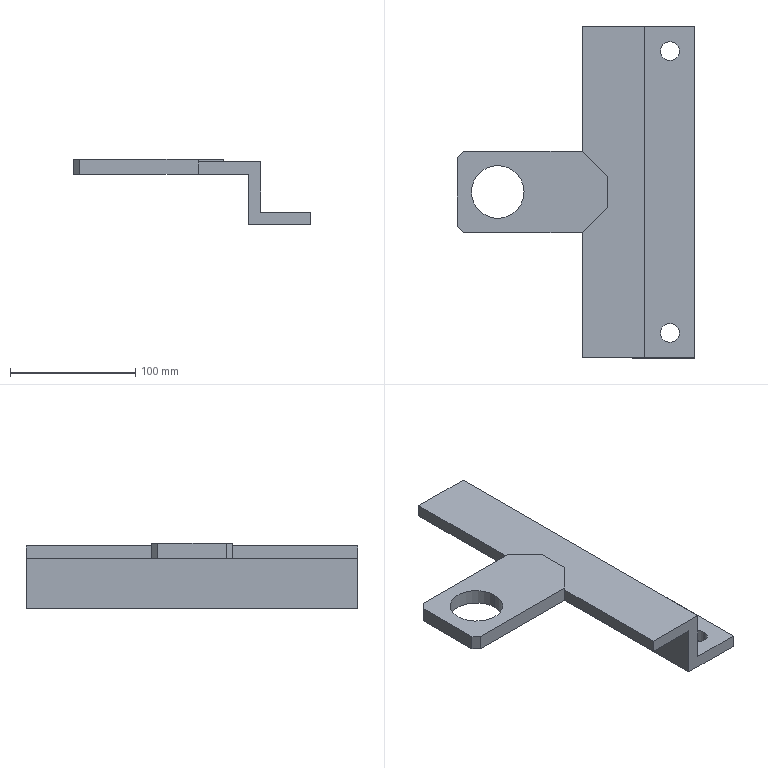Part | SolidWorks | features ICE 4, Chamfer 2, Extrusion 1 | 1 solid | 26 faces | box 190 x 265 x 52 mm | volume 403840 mm3 | plane 20 | cylinder 6 | commonest cylinder face diameters 15 x4 42 x2
STEP:
#1=CARTESIAN_POINT('',(130.,112.5,-40.));
#2=VERTEX_POINT('',#1);
#3=CARTESIAN_POINT('',(145.,112.5,-40.));
#4=VERTEX_POINT('',#3);
#5=CARTESIAN_POINT('',(137.5,112.5,-40.));
#6=DIRECTION('',(0.,0.,1.));
#7=DIRECTION('',(1.,0.,0.));
#8=AXIS2_PLACEMENT_3D('',#5,#6,#7);
#9=CIRCLE('',#8,7.5);
#10=EDGE_CURVE('',#2,#4,#9,.T.);
#11=ORIENTED_EDGE('',*,*,#10,.F.);
#12=CARTESIAN_POINT('',(130.,112.5,-30.));
#13=VERTEX_POINT('',#12);
#14=CARTESIAN_POINT('',(130.,112.5,-40.));
#15=DIRECTION('',(0.,0.,1.));
#16=VECTOR('',#15,1000.);
#17=LINE('',#14,#16);
#18=EDGE_CURVE('',#2,#13,#17,.T.);
#19=ORIENTED_EDGE('',*,*,#18,.T.);
#20=CARTESIAN_POINT('',(145.,112.5,-30.));
#21=VERTEX_POINT('',#20);
#22=CARTESIAN_POINT('',(137.5,112.5,-30.));
#23=DIRECTION('',(0.,0.,1.));
#24=DIRECTION('',(1.,0.,0.));
#25=AXIS2_PLACEMENT_3D('',#22,#23,#24);
#26=CIRCLE('',#25,7.5);
#27=EDGE_CURVE('',#13,#21,#26,.T.);
#28=ORIENTED_EDGE('',*,*,#27,.T.);
#29=CARTESIAN_POINT('',(145.,112.5,-40.));
#30=DIRECTION('',(0.,0.,1.));
#31=VECTOR('',#30,1000.);
#32=LINE('',#29,#31);
#33=EDGE_CURVE('',#4,#21,#32,.T.);
#34=ORIENTED_EDGE('',*,*,#33,.F.);
#35=EDGE_LOOP('',(#11,#19,#28,#34));
#36=FACE_OUTER_BOUND('',#35,.T.);
#37=CARTESIAN_POINT('',(137.5,112.5,-40.));
#38=DIRECTION('',(0.,0.,1.));
#39=DIRECTION('',(1.,0.,0.));
#40=AXIS2_PLACEMENT_3D('',#37,#38,#39);
#41=CYLINDRICAL_SURFACE('',#40,7.5);
#42=ADVANCED_FACE('',(#36),#41,.F.);
#43=CARTESIAN_POINT('',(130.,-112.5,-40.));
#44=VERTEX_POINT('',#43);
#45=CARTESIAN_POINT('',(145.,-112.5,-40.));
#46=VERTEX_POINT('',#45);
#47=CARTESIAN_POINT('',(137.5,-112.5,-40.));
#48=DIRECTION('',(0.,0.,1.));
#49=DIRECTION('',(1.,0.,0.));
#50=AXIS2_PLACEMENT_3D('',#47,#48,#49);
#51=CIRCLE('',#50,7.5);
#52=EDGE_CURVE('',#44,#46,#51,.T.);
#53=ORIENTED_EDGE('',*,*,#52,.F.);
#54=CARTESIAN_POINT('',(130.,-112.5,-30.));
#55=VERTEX_POINT('',#54);
#56=CARTESIAN_POINT('',(130.,-112.5,-40.));
#57=DIRECTION('',(0.,0.,1.));
#58=VECTOR('',#57,1000.);
#59=LINE('',#56,#58);
#60=EDGE_CURVE('',#44,#55,#59,.T.);
#61=ORIENTED_EDGE('',*,*,#60,.T.);
#62=CARTESIAN_POINT('',(145.,-112.5,-30.));
#63=VERTEX_POINT('',#62);
#64=CARTESIAN_POINT('',(137.5,-112.5,-30.));
#65=DIRECTION('',(0.,0.,1.));
#66=DIRECTION('',(1.,0.,0.));
#67=AXIS2_PLACEMENT_3D('',#64,#65,#66);
#68=CIRCLE('',#67,7.5);
#69=EDGE_CURVE('',#55,#63,#68,.T.);
#70=ORIENTED_EDGE('',*,*,#69,.T.);
#71=CARTESIAN_POINT('',(145.,-112.5,-40.));
#72=DIRECTION('',(0.,0.,1.));
#73=VECTOR('',#72,1000.);
#74=LINE('',#71,#73);
#75=EDGE_CURVE('',#46,#63,#74,.T.);
#76=ORIENTED_EDGE('',*,*,#75,.F.);
#77=EDGE_LOOP('',(#53,#61,#70,#76));
#78=FACE_OUTER_BOUND('',#77,.T.);
#79=CARTESIAN_POINT('',(137.5,-112.5,-40.));
#80=DIRECTION('',(0.,0.,1.));
#81=DIRECTION('',(1.,0.,0.));
#82=AXIS2_PLACEMENT_3D('',#79,#80,#81);
#83=CYLINDRICAL_SURFACE('',#82,7.5);
#84=ADVANCED_FACE('',(#78),#83,.F.);
#85=CARTESIAN_POINT('',(-21.,0.,12.));
#86=VERTEX_POINT('',#85);
#87=CARTESIAN_POINT('',(21.,0.,12.));
#88=VERTEX_POINT('',#87);
#89=CARTESIAN_POINT('',(0.,0.,12.));
#90=DIRECTION('',(0.,0.,1.));
#91=DIRECTION('',(1.,0.,0.));
#92=AXIS2_PLACEMENT_3D('',#89,#90,#91);
#93=CIRCLE('',#92,21.);
#94=EDGE_CURVE('',#86,#88,#93,.T.);
#95=ORIENTED_EDGE('',*,*,#94,.T.);
#96=CARTESIAN_POINT('',(21.,0.,0.));
#97=VERTEX_POINT('',#96);
#98=CARTESIAN_POINT('',(21.,0.,12.));
#99=DIRECTION('',(0.,0.,-1.));
#100=VECTOR('',#99,1000.);
#101=LINE('',#98,#100);
#102=EDGE_CURVE('',#88,#97,#101,.T.);
#103=ORIENTED_EDGE('',*,*,#102,.T.);
#104=CARTESIAN_POINT('',(-21.,0.,0.));
#105=VERTEX_POINT('',#104);
#106=CARTESIAN_POINT('',(0.,0.,0.));
#107=DIRECTION('',(0.,0.,1.));
#108=DIRECTION('',(1.,0.,0.));
#109=AXIS2_PLACEMENT_3D('',#106,#107,#108);
#110=CIRCLE('',#109,21.);
#111=EDGE_CURVE('',#105,#97,#110,.T.);
#112=ORIENTED_EDGE('',*,*,#111,.F.);
#113=CARTESIAN_POINT('',(-21.,0.,12.));
#114=DIRECTION('',(0.,0.,-1.));
#115=VECTOR('',#114,1000.);
#116=LINE('',#113,#115);
#117=EDGE_CURVE('',#86,#105,#116,.T.);
#118=ORIENTED_EDGE('',*,*,#117,.F.);
#119=EDGE_LOOP('',(#95,#103,#112,#118));
#120=FACE_OUTER_BOUND('',#119,.T.);
#121=CARTESIAN_POINT('',(0.,0.,12.));
#122=DIRECTION('',(0.,0.,-1.));
#123=DIRECTION('',(-1.,0.,0.));
#124=AXIS2_PLACEMENT_3D('',#121,#122,#123);
#125=CYLINDRICAL_SURFACE('',#124,21.);
#126=ADVANCED_FACE('',(#120),#125,.F.);
#127=CARTESIAN_POINT('',(117.5,-132.5,10.));
#128=VERTEX_POINT('',#127);
#129=CARTESIAN_POINT('',(117.5,-132.5,-30.));
#130=VERTEX_POINT('',#129);
#131=CARTESIAN_POINT('',(117.5,-132.5,10.));
#132=DIRECTION('',(0.,0.,-1.));
#133=VECTOR('',#132,1000.);
#134=LINE('',#131,#133);
#135=EDGE_CURVE('',#128,#130,#134,.T.);
#136=ORIENTED_EDGE('',*,*,#135,.T.);
#137=CARTESIAN_POINT('',(117.5,132.5,-30.));
#138=VERTEX_POINT('',#137);
#139=CARTESIAN_POINT('',(117.5,-132.5,-30.));
#140=DIRECTION('',(0.,1.,0.));
#141=VECTOR('',#140,1000.);
#142=LINE('',#139,#141);
#143=EDGE_CURVE('',#130,#138,#142,.T.);
#144=ORIENTED_EDGE('',*,*,#143,.T.);
#145=CARTESIAN_POINT('',(117.5,132.5,10.));
#146=VERTEX_POINT('',#145);
#147=CARTESIAN_POINT('',(117.5,132.5,10.));
#148=DIRECTION('',(0.,0.,-1.));
#149=VECTOR('',#148,1000.);
#150=LINE('',#147,#149);
#151=EDGE_CURVE('',#146,#138,#150,.T.);
#152=ORIENTED_EDGE('',*,*,#151,.F.);
#153=CARTESIAN_POINT('',(117.5,-132.5,10.));
#154=DIRECTION('',(0.,-1.,0.));
#155=VECTOR('',#154,1000.);
#156=LINE('',#153,#155);
#157=EDGE_CURVE('',#146,#128,#156,.T.);
#158=ORIENTED_EDGE('',*,*,#157,.T.);
#159=EDGE_LOOP('',(#136,#144,#152,#158));
#160=FACE_OUTER_BOUND('',#159,.T.);
#161=CARTESIAN_POINT('',(117.5,-132.5,10.));
#162=DIRECTION('',(1.,0.,0.));
#163=DIRECTION('',(0.,0.,-1.));
#164=AXIS2_PLACEMENT_3D('',#161,#162,#163);
#165=PLANE('',#164);
#166=ADVANCED_FACE('',(#160),#165,.T.);
#167=CARTESIAN_POINT('',(87.5,-12.5,12.));
#168=VERTEX_POINT('',#167);
#169=CARTESIAN_POINT('',(87.5,12.5,12.));
#170=VERTEX_POINT('',#169);
#171=CARTESIAN_POINT('',(87.5,32.5,12.));
#172=DIRECTION('',(0.,1.,0.));
#173=VECTOR('',#172,1000.);
#174=LINE('',#171,#173);
#175=EDGE_CURVE('',#168,#170,#174,.T.);
#176=ORIENTED_EDGE('',*,*,#175,.T.);
#177=CARTESIAN_POINT('',(67.5,32.5,12.));
#178=VERTEX_POINT('',#177);
#179=CARTESIAN_POINT('',(50.,50.,12.));
#180=DIRECTION('',(-0.7071,0.7071,0.));
#181=VECTOR('',#180,1000.);
#182=LINE('',#179,#181);
#183=EDGE_CURVE('',#170,#178,#182,.T.);
#184=ORIENTED_EDGE('',*,*,#183,.T.);
#185=CARTESIAN_POINT('',(-27.5,32.5,12.));
#186=VERTEX_POINT('',#185);
#187=CARTESIAN_POINT('',(32.5,32.5,12.));
#188=DIRECTION('',(-1.,0.,0.));
#189=VECTOR('',#188,1000.);
#190=LINE('',#187,#189);
#191=EDGE_CURVE('',#178,#186,#190,.T.);
#192=ORIENTED_EDGE('',*,*,#191,.T.);
#193=CARTESIAN_POINT('',(-32.5,27.5,12.));
#194=VERTEX_POINT('',#193);
#195=CARTESIAN_POINT('',(-30.,30.,12.));
#196=DIRECTION('',(-0.7071,-0.7071,0.));
#197=VECTOR('',#196,1000.);
#198=LINE('',#195,#197);
#199=EDGE_CURVE('',#186,#194,#198,.T.);
#200=ORIENTED_EDGE('',*,*,#199,.T.);
#201=CARTESIAN_POINT('',(-32.5,-27.5,12.));
#202=VERTEX_POINT('',#201);
#203=CARTESIAN_POINT('',(-32.5,32.5,12.));
#204=DIRECTION('',(0.,-1.,0.));
#205=VECTOR('',#204,1000.);
#206=LINE('',#203,#205);
#207=EDGE_CURVE('',#194,#202,#206,.T.);
#208=ORIENTED_EDGE('',*,*,#207,.T.);
#209=CARTESIAN_POINT('',(-27.5,-32.5,12.));
#210=VERTEX_POINT('',#209);
#211=CARTESIAN_POINT('',(-30.,-30.,12.));
#212=DIRECTION('',(0.7071,-0.7071,0.));
#213=VECTOR('',#212,1000.);
#214=LINE('',#211,#213);
#215=EDGE_CURVE('',#202,#210,#214,.T.);
#216=ORIENTED_EDGE('',*,*,#215,.T.);
#217=CARTESIAN_POINT('',(67.5,-32.5,12.));
#218=VERTEX_POINT('',#217);
#219=CARTESIAN_POINT('',(87.5,-32.5,12.));
#220=DIRECTION('',(1.,0.,0.));
#221=VECTOR('',#220,1000.);
#222=LINE('',#219,#221);
#223=EDGE_CURVE('',#210,#218,#222,.T.);
#224=ORIENTED_EDGE('',*,*,#223,.T.);
#225=CARTESIAN_POINT('',(50.,-50.,12.));
#226=DIRECTION('',(0.7071,0.7071,0.));
#227=VECTOR('',#226,1000.);
#228=LINE('',#225,#227);
#229=EDGE_CURVE('',#218,#168,#228,.T.);
#230=ORIENTED_EDGE('',*,*,#229,.T.);
#231=EDGE_LOOP('',(#176,#184,#192,#200,#208,#216,#224,#230));
#232=FACE_OUTER_BOUND('',#231,.T.);
#233=ORIENTED_EDGE('',*,*,#94,.F.);
#234=CARTESIAN_POINT('',(0.,0.,12.));
#235=DIRECTION('',(0.,0.,1.));
#236=DIRECTION('',(1.,0.,0.));
#237=AXIS2_PLACEMENT_3D('',#234,#235,#236);
#238=CIRCLE('',#237,21.);
#239=EDGE_CURVE('',#88,#86,#238,.T.);
#240=ORIENTED_EDGE('',*,*,#239,.F.);
#241=EDGE_LOOP('',(#233,#240));
#242=FACE_BOUND('',#241,.T.);
#243=CARTESIAN_POINT('',(0.,0.,12.));
#244=DIRECTION('',(0.,0.,1.));
#245=DIRECTION('',(1.,0.,0.));
#246=AXIS2_PLACEMENT_3D('',#243,#244,#245);
#247=PLANE('',#246);
#248=ADVANCED_FACE('',(#232,#242),#247,.T.);
#249=CARTESIAN_POINT('',(67.5,132.5,0.));
#250=VERTEX_POINT('',#249);
#251=CARTESIAN_POINT('',(107.5,132.5,0.));
#252=VERTEX_POINT('',#251);
#253=CARTESIAN_POINT('',(117.5,132.5,0.));
#254=DIRECTION('',(1.,0.,0.));
#255=VECTOR('',#254,1000.);
#256=LINE('',#253,#255);
#257=EDGE_CURVE('',#250,#252,#256,.T.);
#258=ORIENTED_EDGE('',*,*,#257,.T.);
#259=CARTESIAN_POINT('',(107.5,-132.5,0.));
#260=VERTEX_POINT('',#259);
#261=CARTESIAN_POINT('',(107.5,0.,0.));
#262=DIRECTION('',(0.,-1.,0.));
#263=VECTOR('',#262,1000.);
#264=LINE('',#261,#263);
#265=EDGE_CURVE('',#252,#260,#264,.T.);
#266=ORIENTED_EDGE('',*,*,#265,.T.);
#267=CARTESIAN_POINT('',(67.5,-132.5,0.));
#268=VERTEX_POINT('',#267);
#269=CARTESIAN_POINT('',(67.5,-132.5,0.));
#270=DIRECTION('',(-1.,0.,0.));
#271=VECTOR('',#270,1000.);
#272=LINE('',#269,#271);
#273=EDGE_CURVE('',#260,#268,#272,.T.);
#274=ORIENTED_EDGE('',*,*,#273,.T.);
#275=CARTESIAN_POINT('',(67.5,-32.5,0.));
#276=VERTEX_POINT('',#275);
#277=CARTESIAN_POINT('',(67.5,-32.5,0.));
#278=DIRECTION('',(0.,1.,0.));
#279=VECTOR('',#278,1000.);
#280=LINE('',#277,#279);
#281=EDGE_CURVE('',#268,#276,#280,.T.);
#282=ORIENTED_EDGE('',*,*,#281,.T.);
#283=CARTESIAN_POINT('',(-27.5,-32.5,0.));
#284=VERTEX_POINT('',#283);
#285=CARTESIAN_POINT('',(-32.5,-32.5,0.));
#286=DIRECTION('',(1.,0.,0.));
#287=VECTOR('',#286,1000.);
#288=LINE('',#285,#287);
#289=EDGE_CURVE('',#284,#276,#288,.T.);
#290=ORIENTED_EDGE('',*,*,#289,.F.);
#291=CARTESIAN_POINT('',(-32.5,-27.5,0.));
#292=VERTEX_POINT('',#291);
#293=CARTESIAN_POINT('',(-27.5,-32.5,0.));
#294=DIRECTION('',(-0.7071,0.7071,0.));
#295=VECTOR('',#294,1000.);
#296=LINE('',#293,#295);
#297=EDGE_CURVE('',#284,#292,#296,.T.);
#298=ORIENTED_EDGE('',*,*,#297,.T.);
#299=CARTESIAN_POINT('',(-32.5,27.5,0.));
#300=VERTEX_POINT('',#299);
#301=CARTESIAN_POINT('',(-32.5,32.5,0.));
#302=DIRECTION('',(0.,-1.,0.));
#303=VECTOR('',#302,1000.);
#304=LINE('',#301,#303);
#305=EDGE_CURVE('',#300,#292,#304,.T.);
#306=ORIENTED_EDGE('',*,*,#305,.F.);
#307=CARTESIAN_POINT('',(-27.5,32.5,0.));
#308=VERTEX_POINT('',#307);
#309=CARTESIAN_POINT('',(-32.5,27.5,0.));
#310=DIRECTION('',(0.7071,0.7071,0.));
#311=VECTOR('',#310,1000.);
#312=LINE('',#309,#311);
#313=EDGE_CURVE('',#300,#308,#312,.T.);
#314=ORIENTED_EDGE('',*,*,#313,.T.);
#315=CARTESIAN_POINT('',(67.5,32.5,0.));
#316=VERTEX_POINT('',#315);
#317=CARTESIAN_POINT('',(-32.5,32.5,0.));
#318=DIRECTION('',(-1.,0.,0.));
#319=VECTOR('',#318,1000.);
#320=LINE('',#317,#319);
#321=EDGE_CURVE('',#316,#308,#320,.T.);
#322=ORIENTED_EDGE('',*,*,#321,.F.);
#323=CARTESIAN_POINT('',(67.5,132.5,0.));
#324=DIRECTION('',(0.,1.,0.));
#325=VECTOR('',#324,1000.);
#326=LINE('',#323,#325);
#327=EDGE_CURVE('',#316,#250,#326,.T.);
#328=ORIENTED_EDGE('',*,*,#327,.T.);
#329=EDGE_LOOP('',(#258,#266,#274,#282,#290,#298,#306,#314,#322,#328));
#330=FACE_OUTER_BOUND('',#329,.T.);
#331=ORIENTED_EDGE('',*,*,#111,.T.);
#332=CARTESIAN_POINT('',(0.,0.,0.));
#333=DIRECTION('',(0.,0.,1.));
#334=DIRECTION('',(1.,0.,0.));
#335=AXIS2_PLACEMENT_3D('',#332,#333,#334);
#336=CIRCLE('',#335,21.);
#337=EDGE_CURVE('',#97,#105,#336,.T.);
#338=ORIENTED_EDGE('',*,*,#337,.T.);
#339=EDGE_LOOP('',(#331,#338));
#340=FACE_BOUND('',#339,.T.);
#341=CARTESIAN_POINT('',(0.,0.,0.));
#342=DIRECTION('',(0.,0.,1.));
#343=DIRECTION('',(1.,0.,0.));
#344=AXIS2_PLACEMENT_3D('',#341,#342,#343);
#345=PLANE('',#344);
#346=ADVANCED_FACE('',(#330,#340),#345,.F.);
#347=CARTESIAN_POINT('',(87.5,-12.5,10.));
#348=VERTEX_POINT('',#347);
#349=CARTESIAN_POINT('',(87.5,-12.5,12.));
#350=DIRECTION('',(0.,0.,-1.));
#351=VECTOR('',#350,1000.);
#352=LINE('',#349,#351);
#353=EDGE_CURVE('',#168,#348,#352,.T.);
#354=ORIENTED_EDGE('',*,*,#353,.T.);
#355=CARTESIAN_POINT('',(87.5,12.5,10.));
#356=VERTEX_POINT('',#355);
#357=CARTESIAN_POINT('',(87.5,-12.5,10.));
#358=DIRECTION('',(0.,1.,0.));
#359=VECTOR('',#358,1000.);
#360=LINE('',#357,#359);
#361=EDGE_CURVE('',#348,#356,#360,.T.);
#362=ORIENTED_EDGE('',*,*,#361,.T.);
#363=CARTESIAN_POINT('',(87.5,12.5,12.));
#364=DIRECTION('',(0.,0.,1.));
#365=VECTOR('',#364,1000.);
#366=LINE('',#363,#365);
#367=EDGE_CURVE('',#356,#170,#366,.T.);
#368=ORIENTED_EDGE('',*,*,#367,.T.);
#369=ORIENTED_EDGE('',*,*,#175,.F.);
#370=EDGE_LOOP('',(#354,#362,#368,#369));
#371=FACE_OUTER_BOUND('',#370,.T.);
#372=CARTESIAN_POINT('',(87.5,32.5,12.));
#373=DIRECTION('',(-1.,0.,0.));
#374=DIRECTION('',(0.,-1.,0.));
#375=AXIS2_PLACEMENT_3D('',#372,#373,#374);
#376=PLANE('',#375);
#377=ADVANCED_FACE('',(#371),#376,.F.);
#378=ORIENTED_EDGE('',*,*,#191,.F.);
#379=CARTESIAN_POINT('',(67.5,32.5,10.));
#380=VERTEX_POINT('',#379);
#381=CARTESIAN_POINT('',(67.5,32.5,12.));
#382=DIRECTION('',(0.,0.,-1.));
#383=VECTOR('',#382,1000.);
#384=LINE('',#381,#383);
#385=EDGE_CURVE('',#178,#380,#384,.T.);
#386=ORIENTED_EDGE('',*,*,#385,.T.);
#387=CARTESIAN_POINT('',(67.5,32.5,10.));
#388=DIRECTION('',(0.,0.,-1.));
#389=VECTOR('',#388,1000.);
#390=LINE('',#387,#389);
#391=EDGE_CURVE('',#380,#316,#390,.T.);
#392=ORIENTED_EDGE('',*,*,#391,.T.);
#393=ORIENTED_EDGE('',*,*,#321,.T.);
#394=CARTESIAN_POINT('',(-27.5,32.5,12.));
#395=DIRECTION('',(0.,0.,1.));
#396=VECTOR('',#395,1000.);
#397=LINE('',#394,#396);
#398=EDGE_CURVE('',#308,#186,#397,.T.);
#399=ORIENTED_EDGE('',*,*,#398,.T.);
#400=EDGE_LOOP('',(#378,#386,#392,#393,#399));
#401=FACE_OUTER_BOUND('',#400,.T.);
#402=CARTESIAN_POINT('',(-32.5,32.5,12.));
#403=DIRECTION('',(0.,-1.,0.));
#404=DIRECTION('',(0.,0.,-1.));
#405=AXIS2_PLACEMENT_3D('',#402,#403,#404);
#406=PLANE('',#405);
#407=ADVANCED_FACE('',(#401),#406,.F.);
#408=ORIENTED_EDGE('',*,*,#305,.T.);
#409=CARTESIAN_POINT('',(-32.5,-27.5,12.));
#410=DIRECTION('',(0.,0.,1.));
#411=VECTOR('',#410,1000.);
#412=LINE('',#409,#411);
#413=EDGE_CURVE('',#292,#202,#412,.T.);
#414=ORIENTED_EDGE('',*,*,#413,.T.);
#415=ORIENTED_EDGE('',*,*,#207,.F.);
#416=CARTESIAN_POINT('',(-32.5,27.5,12.));
#417=DIRECTION('',(0.,0.,-1.));
#418=VECTOR('',#417,1000.);
#419=LINE('',#416,#418);
#420=EDGE_CURVE('',#194,#300,#419,.T.);
#421=ORIENTED_EDGE('',*,*,#420,.T.);
#422=EDGE_LOOP('',(#408,#414,#415,#421));
#423=FACE_OUTER_BOUND('',#422,.T.);
#424=CARTESIAN_POINT('',(-32.5,32.5,12.));
#425=DIRECTION('',(1.,0.,0.));
#426=DIRECTION('',(0.,1.,0.));
#427=AXIS2_PLACEMENT_3D('',#424,#425,#426);
#428=PLANE('',#427);
#429=ADVANCED_FACE('',(#423),#428,.F.);
#430=ORIENTED_EDGE('',*,*,#289,.T.);
#431=CARTESIAN_POINT('',(67.5,-32.5,10.));
#432=VERTEX_POINT('',#431);
#433=CARTESIAN_POINT('',(67.5,-32.5,12.));
#434=DIRECTION('',(0.,0.,1.));
#435=VECTOR('',#434,1000.);
#436=LINE('',#433,#435);
#437=EDGE_CURVE('',#276,#432,#436,.T.);
#438=ORIENTED_EDGE('',*,*,#437,.T.);
#439=CARTESIAN_POINT('',(67.5,-32.5,12.));
#440=DIRECTION('',(0.,0.,1.));
#441=VECTOR('',#440,1000.);
#442=LINE('',#439,#441);
#443=EDGE_CURVE('',#432,#218,#442,.T.);
#444=ORIENTED_EDGE('',*,*,#443,.T.);
#445=ORIENTED_EDGE('',*,*,#223,.F.);
#446=CARTESIAN_POINT('',(-27.5,-32.5,12.));
#447=DIRECTION('',(0.,0.,-1.));
#448=VECTOR('',#447,1000.);
#449=LINE('',#446,#448);
#450=EDGE_CURVE('',#210,#284,#449,.T.);
#451=ORIENTED_EDGE('',*,*,#450,.T.);
#452=EDGE_LOOP('',(#430,#438,#444,#445,#451));
#453=FACE_OUTER_BOUND('',#452,.T.);
#454=CARTESIAN_POINT('',(-32.5,-32.5,12.));
#455=DIRECTION('',(0.,1.,0.));
#456=DIRECTION('',(0.,0.,1.));
#457=AXIS2_PLACEMENT_3D('',#454,#455,#456);
#458=PLANE('',#457);
#459=ADVANCED_FACE('',(#453),#458,.F.);
#460=ORIENTED_EDGE('',*,*,#102,.F.);
#461=ORIENTED_EDGE('',*,*,#239,.T.);
#462=ORIENTED_EDGE('',*,*,#117,.T.);
#463=ORIENTED_EDGE('',*,*,#337,.F.);
#464=EDGE_LOOP('',(#460,#461,#462,#463));
#465=FACE_OUTER_BOUND('',#464,.T.);
#466=CARTESIAN_POINT('',(0.,0.,12.));
#467=DIRECTION('',(0.,0.,-1.));
#468=DIRECTION('',(-1.,0.,0.));
#469=AXIS2_PLACEMENT_3D('',#466,#467,#468);
#470=CYLINDRICAL_SURFACE('',#469,21.);
#471=ADVANCED_FACE('',(#465),#470,.F.);
#472=ORIENTED_EDGE('',*,*,#215,.F.);
#473=ORIENTED_EDGE('',*,*,#413,.F.);
#474=ORIENTED_EDGE('',*,*,#297,.F.);
#475=ORIENTED_EDGE('',*,*,#450,.F.);
#476=EDGE_LOOP('',(#472,#473,#474,#475));
#477=FACE_OUTER_BOUND('',#476,.T.);
#478=CARTESIAN_POINT('',(-27.5,-32.5,12.));
#479=DIRECTION('',(0.7071,0.7071,0.));
#480=DIRECTION('',(0.,0.,-1.));
#481=AXIS2_PLACEMENT_3D('',#478,#479,#480);
#482=PLANE('',#481);
#483=ADVANCED_FACE('',(#477),#482,.F.);
#484=ORIENTED_EDGE('',*,*,#199,.F.);
#485=ORIENTED_EDGE('',*,*,#398,.F.);
#486=ORIENTED_EDGE('',*,*,#313,.F.);
#487=ORIENTED_EDGE('',*,*,#420,.F.);
#488=EDGE_LOOP('',(#484,#485,#486,#487));
#489=FACE_OUTER_BOUND('',#488,.T.);
#490=CARTESIAN_POINT('',(-32.5,27.5,12.));
#491=DIRECTION('',(0.7071,-0.7071,0.));
#492=DIRECTION('',(0.,0.,-1.));
#493=AXIS2_PLACEMENT_3D('',#490,#491,#492);
#494=PLANE('',#493);
#495=ADVANCED_FACE('',(#489),#494,.F.);
#496=CARTESIAN_POINT('',(67.5,32.5,10.));
#497=DIRECTION('',(-0.7071,0.7071,0.));
#498=VECTOR('',#497,1000.);
#499=LINE('',#496,#498);
#500=EDGE_CURVE('',#356,#380,#499,.T.);
#501=ORIENTED_EDGE('',*,*,#500,.T.);
#502=ORIENTED_EDGE('',*,*,#385,.F.);
#503=ORIENTED_EDGE('',*,*,#183,.F.);
#504=ORIENTED_EDGE('',*,*,#367,.F.);
#505=EDGE_LOOP('',(#501,#502,#503,#504));
#506=FACE_OUTER_BOUND('',#505,.T.);
#507=CARTESIAN_POINT('',(67.5,32.5,12.));
#508=DIRECTION('',(-0.7071,-0.7071,0.));
#509=DIRECTION('',(0.,0.,-1.));
#510=AXIS2_PLACEMENT_3D('',#507,#508,#509);
#511=PLANE('',#510);
#512=ADVANCED_FACE('',(#506),#511,.F.);
#513=CARTESIAN_POINT('',(87.5,-12.5,10.));
#514=DIRECTION('',(0.7071,0.7071,0.));
#515=VECTOR('',#514,1000.);
#516=LINE('',#513,#515);
#517=EDGE_CURVE('',#432,#348,#516,.T.);
#518=ORIENTED_EDGE('',*,*,#517,.T.);
#519=ORIENTED_EDGE('',*,*,#353,.F.);
#520=ORIENTED_EDGE('',*,*,#229,.F.);
#521=ORIENTED_EDGE('',*,*,#443,.F.);
#522=EDGE_LOOP('',(#518,#519,#520,#521));
#523=FACE_OUTER_BOUND('',#522,.T.);
#524=CARTESIAN_POINT('',(87.5,-12.5,12.));
#525=DIRECTION('',(-0.7071,0.7071,0.));
#526=DIRECTION('',(0.,0.,-1.));
#527=AXIS2_PLACEMENT_3D('',#524,#525,#526);
#528=PLANE('',#527);
#529=ADVANCED_FACE('',(#523),#528,.F.);
#530=ORIENTED_EDGE('',*,*,#327,.F.);
#531=ORIENTED_EDGE('',*,*,#391,.F.);
#532=CARTESIAN_POINT('',(67.5,132.5,10.));
#533=VERTEX_POINT('',#532);
#534=CARTESIAN_POINT('',(67.5,132.5,10.));
#535=DIRECTION('',(0.,1.,0.));
#536=VECTOR('',#535,1000.);
#537=LINE('',#534,#536);
#538=EDGE_CURVE('',#380,#533,#537,.T.);
#539=ORIENTED_EDGE('',*,*,#538,.T.);
#540=CARTESIAN_POINT('',(67.5,132.5,10.));
#541=DIRECTION('',(0.,0.,-1.));
#542=VECTOR('',#541,1000.);
#543=LINE('',#540,#542);
#544=EDGE_CURVE('',#533,#250,#543,.T.);
#545=ORIENTED_EDGE('',*,*,#544,.T.);
#546=EDGE_LOOP('',(#530,#531,#539,#545));
#547=FACE_OUTER_BOUND('',#546,.T.);
#548=CARTESIAN_POINT('',(67.5,132.5,10.));
#549=DIRECTION('',(-1.,0.,0.));
#550=DIRECTION('',(0.,-1.,0.));
#551=AXIS2_PLACEMENT_3D('',#548,#549,#550);
#552=PLANE('',#551);
#553=ADVANCED_FACE('',(#547),#552,.T.);
#554=ORIENTED_EDGE('',*,*,#281,.F.);
#555=CARTESIAN_POINT('',(67.5,-132.5,10.));
#556=VERTEX_POINT('',#555);
#557=CARTESIAN_POINT('',(67.5,-132.5,10.));
#558=DIRECTION('',(0.,0.,-1.));
#559=VECTOR('',#558,1000.);
#560=LINE('',#557,#559);
#561=EDGE_CURVE('',#556,#268,#560,.T.);
#562=ORIENTED_EDGE('',*,*,#561,.F.);
#563=CARTESIAN_POINT('',(67.5,-32.5,10.));
#564=DIRECTION('',(0.,1.,0.));
#565=VECTOR('',#564,1000.);
#566=LINE('',#563,#565);
#567=EDGE_CURVE('',#556,#432,#566,.T.);
#568=ORIENTED_EDGE('',*,*,#567,.T.);
#569=ORIENTED_EDGE('',*,*,#437,.F.);
#570=EDGE_LOOP('',(#554,#562,#568,#569));
#571=FACE_OUTER_BOUND('',#570,.T.);
#572=CARTESIAN_POINT('',(67.5,-32.5,10.));
#573=DIRECTION('',(-1.,0.,0.));
#574=DIRECTION('',(0.,-1.,0.));
#575=AXIS2_PLACEMENT_3D('',#572,#573,#574);
#576=PLANE('',#575);
#577=ADVANCED_FACE('',(#571),#576,.T.);
#578=CARTESIAN_POINT('',(157.5,-132.5,-30.));
#579=VERTEX_POINT('',#578);
#580=CARTESIAN_POINT('',(107.5,-132.5,-30.));
#581=DIRECTION('',(-1.,0.,0.));
#582=VECTOR('',#581,1000.);
#583=LINE('',#580,#582);
#584=EDGE_CURVE('',#579,#130,#583,.T.);
#585=ORIENTED_EDGE('',*,*,#584,.T.);
#586=ORIENTED_EDGE('',*,*,#135,.F.);
#587=CARTESIAN_POINT('',(67.5,-132.5,10.));
#588=DIRECTION('',(-1.,0.,0.));
#589=VECTOR('',#588,1000.);
#590=LINE('',#587,#589);
#591=EDGE_CURVE('',#128,#556,#590,.T.);
#592=ORIENTED_EDGE('',*,*,#591,.T.);
#593=ORIENTED_EDGE('',*,*,#561,.T.);
#594=ORIENTED_EDGE('',*,*,#273,.F.);
#595=CARTESIAN_POINT('',(107.5,-132.5,-40.));
#596=VERTEX_POINT('',#595);
#597=CARTESIAN_POINT('',(107.5,-132.5,-40.));
#598=DIRECTION('',(0.,0.,1.));
#599=VECTOR('',#598,1000.);
#600=LINE('',#597,#599);
#601=EDGE_CURVE('',#596,#260,#600,.T.);
#602=ORIENTED_EDGE('',*,*,#601,.F.);
#603=CARTESIAN_POINT('',(157.5,-132.5,-40.));
#604=VERTEX_POINT('',#603);
#605=CARTESIAN_POINT('',(117.5,-132.5,-40.));
#606=DIRECTION('',(1.,0.,0.));
#607=VECTOR('',#606,1000.);
#608=LINE('',#605,#607);
#609=EDGE_CURVE('',#596,#604,#608,.T.);
#610=ORIENTED_EDGE('',*,*,#609,.T.);
#611=CARTESIAN_POINT('',(157.5,-132.5,-30.));
#612=DIRECTION('',(0.,0.,-1.));
#613=VECTOR('',#612,1000.);
#614=LINE('',#611,#613);
#615=EDGE_CURVE('',#579,#604,#614,.T.);
#616=ORIENTED_EDGE('',*,*,#615,.F.);
#617=EDGE_LOOP('',(#585,#586,#592,#593,#594,#602,#610,#616));
#618=FACE_OUTER_BOUND('',#617,.T.);
#619=CARTESIAN_POINT('',(67.5,-132.5,10.));
#620=DIRECTION('',(0.,-1.,0.));
#621=DIRECTION('',(0.,0.,-1.));
#622=AXIS2_PLACEMENT_3D('',#619,#620,#621);
#623=PLANE('',#622);
#624=ADVANCED_FACE('',(#618),#623,.T.);
#625=CARTESIAN_POINT('',(107.5,132.5,-40.));
#626=VERTEX_POINT('',#625);
#627=CARTESIAN_POINT('',(107.5,132.5,-40.));
#628=DIRECTION('',(0.,0.,1.));
#629=VECTOR('',#628,1000.);
#630=LINE('',#627,#629);
#631=EDGE_CURVE('',#626,#252,#630,.T.);
#632=ORIENTED_EDGE('',*,*,#631,.T.);
#633=ORIENTED_EDGE('',*,*,#257,.F.);
#634=ORIENTED_EDGE('',*,*,#544,.F.);
#635=CARTESIAN_POINT('',(117.5,132.5,10.));
#636=DIRECTION('',(1.,0.,0.));
#637=VECTOR('',#636,1000.);
#638=LINE('',#635,#637);
#639=EDGE_CURVE('',#533,#146,#638,.T.);
#640=ORIENTED_EDGE('',*,*,#639,.T.);
#641=ORIENTED_EDGE('',*,*,#151,.T.);
#642=CARTESIAN_POINT('',(157.5,132.5,-30.));
#643=VERTEX_POINT('',#642);
#644=CARTESIAN_POINT('',(107.5,132.5,-30.));
#645=DIRECTION('',(1.,0.,0.));
#646=VECTOR('',#645,1000.);
#647=LINE('',#644,#646);
#648=EDGE_CURVE('',#138,#643,#647,.T.);
#649=ORIENTED_EDGE('',*,*,#648,.T.);
#650=CARTESIAN_POINT('',(157.5,132.5,-40.));
#651=VERTEX_POINT('',#650);
#652=CARTESIAN_POINT('',(157.5,132.5,-30.));
#653=DIRECTION('',(0.,0.,-1.));
#654=VECTOR('',#653,1000.);
#655=LINE('',#652,#654);
#656=EDGE_CURVE('',#643,#651,#655,.T.);
#657=ORIENTED_EDGE('',*,*,#656,.T.);
#658=CARTESIAN_POINT('',(117.5,132.5,-40.));
#659=DIRECTION('',(-1.,0.,0.));
#660=VECTOR('',#659,1000.);
#661=LINE('',#658,#660);
#662=EDGE_CURVE('',#651,#626,#661,.T.);
#663=ORIENTED_EDGE('',*,*,#662,.T.);
#664=EDGE_LOOP('',(#632,#633,#634,#640,#641,#649,#657,#663));
#665=FACE_OUTER_BOUND('',#664,.T.);
#666=CARTESIAN_POINT('',(117.5,132.5,10.));
#667=DIRECTION('',(0.,1.,0.));
#668=DIRECTION('',(0.,0.,1.));
#669=AXIS2_PLACEMENT_3D('',#666,#667,#668);
#670=PLANE('',#669);
#671=ADVANCED_FACE('',(#665),#670,.T.);
#672=ORIENTED_EDGE('',*,*,#567,.F.);
#673=ORIENTED_EDGE('',*,*,#591,.F.);
#674=ORIENTED_EDGE('',*,*,#157,.F.);
#675=ORIENTED_EDGE('',*,*,#639,.F.);
#676=ORIENTED_EDGE('',*,*,#538,.F.);
#677=ORIENTED_EDGE('',*,*,#500,.F.);
#678=ORIENTED_EDGE('',*,*,#361,.F.);
#679=ORIENTED_EDGE('',*,*,#517,.F.);
#680=EDGE_LOOP('',(#672,#673,#674,#675,#676,#677,#678,#679));
#681=FACE_OUTER_BOUND('',#680,.T.);
#682=CARTESIAN_POINT('',(0.,0.,10.));
#683=DIRECTION('',(0.,0.,1.));
#684=DIRECTION('',(1.,0.,0.));
#685=AXIS2_PLACEMENT_3D('',#682,#683,#684);
#686=PLANE('',#685);
#687=ADVANCED_FACE('',(#681),#686,.T.);
#688=ORIENTED_EDGE('',*,*,#601,.T.);
#689=ORIENTED_EDGE('',*,*,#265,.F.);
#690=ORIENTED_EDGE('',*,*,#631,.F.);
#691=CARTESIAN_POINT('',(107.5,132.5,-40.));
#692=DIRECTION('',(0.,-1.,0.));
#693=VECTOR('',#692,1000.);
#694=LINE('',#691,#693);
#695=EDGE_CURVE('',#626,#596,#694,.T.);
#696=ORIENTED_EDGE('',*,*,#695,.T.);
#697=EDGE_LOOP('',(#688,#689,#690,#696));
#698=FACE_OUTER_BOUND('',#697,.T.);
#699=CARTESIAN_POINT('',(107.5,132.5,-40.));
#700=DIRECTION('',(-1.,0.,0.));
#701=DIRECTION('',(0.,-1.,0.));
#702=AXIS2_PLACEMENT_3D('',#699,#700,#701);
#703=PLANE('',#702);
#704=ADVANCED_FACE('',(#698),#703,.T.);
#705=CARTESIAN_POINT('',(137.5,112.5,-40.));
#706=DIRECTION('',(0.,0.,1.));
#707=DIRECTION('',(1.,0.,0.));
#708=AXIS2_PLACEMENT_3D('',#705,#706,#707);
#709=CIRCLE('',#708,7.5);
#710=EDGE_CURVE('',#4,#2,#709,.T.);
#711=ORIENTED_EDGE('',*,*,#710,.T.);
#712=ORIENTED_EDGE('',*,*,#10,.T.);
#713=EDGE_LOOP('',(#711,#712));
#714=FACE_BOUND('',#713,.T.);
#715=CARTESIAN_POINT('',(137.5,-112.5,-40.));
#716=DIRECTION('',(0.,0.,1.));
#717=DIRECTION('',(1.,0.,0.));
#718=AXIS2_PLACEMENT_3D('',#715,#716,#717);
#719=CIRCLE('',#718,7.5);
#720=EDGE_CURVE('',#46,#44,#719,.T.);
#721=ORIENTED_EDGE('',*,*,#720,.T.);
#722=ORIENTED_EDGE('',*,*,#52,.T.);
#723=EDGE_LOOP('',(#721,#722));
#724=FACE_BOUND('',#723,.T.);
#725=ORIENTED_EDGE('',*,*,#662,.F.);
#726=CARTESIAN_POINT('',(157.5,-132.5,-40.));
#727=DIRECTION('',(0.,-1.,0.));
#728=VECTOR('',#727,1000.);
#729=LINE('',#726,#728);
#730=EDGE_CURVE('',#651,#604,#729,.T.);
#731=ORIENTED_EDGE('',*,*,#730,.T.);
#732=ORIENTED_EDGE('',*,*,#609,.F.);
#733=ORIENTED_EDGE('',*,*,#695,.F.);
#734=EDGE_LOOP('',(#725,#731,#732,#733));
#735=FACE_OUTER_BOUND('',#734,.T.);
#736=CARTESIAN_POINT('',(0.,0.,-40.));
#737=DIRECTION('',(0.,0.,-1.));
#738=DIRECTION('',(-1.,0.,0.));
#739=AXIS2_PLACEMENT_3D('',#736,#737,#738);
#740=PLANE('',#739);
#741=ADVANCED_FACE('',(#714,#724,#735),#740,.T.);
#742=ORIENTED_EDGE('',*,*,#730,.F.);
#743=ORIENTED_EDGE('',*,*,#656,.F.);
#744=CARTESIAN_POINT('',(157.5,-132.5,-30.));
#745=DIRECTION('',(0.,-1.,0.));
#746=VECTOR('',#745,1000.);
#747=LINE('',#744,#746);
#748=EDGE_CURVE('',#643,#579,#747,.T.);
#749=ORIENTED_EDGE('',*,*,#748,.T.);
#750=ORIENTED_EDGE('',*,*,#615,.T.);
#751=EDGE_LOOP('',(#742,#743,#749,#750));
#752=FACE_OUTER_BOUND('',#751,.T.);
#753=CARTESIAN_POINT('',(157.5,-132.5,-30.));
#754=DIRECTION('',(1.,0.,0.));
#755=DIRECTION('',(0.,0.,-1.));
#756=AXIS2_PLACEMENT_3D('',#753,#754,#755);
#757=PLANE('',#756);
#758=ADVANCED_FACE('',(#752),#757,.T.);
#759=CARTESIAN_POINT('',(137.5,112.5,-30.));
#760=DIRECTION('',(0.,0.,1.));
#761=DIRECTION('',(1.,0.,0.));
#762=AXIS2_PLACEMENT_3D('',#759,#760,#761);
#763=CIRCLE('',#762,7.5);
#764=EDGE_CURVE('',#21,#13,#763,.T.);
#765=ORIENTED_EDGE('',*,*,#764,.F.);
#766=ORIENTED_EDGE('',*,*,#27,.F.);
#767=EDGE_LOOP('',(#765,#766));
#768=FACE_BOUND('',#767,.T.);
#769=CARTESIAN_POINT('',(137.5,-112.5,-30.));
#770=DIRECTION('',(0.,0.,1.));
#771=DIRECTION('',(1.,0.,0.));
#772=AXIS2_PLACEMENT_3D('',#769,#770,#771);
#773=CIRCLE('',#772,7.5);
#774=EDGE_CURVE('',#63,#55,#773,.T.);
#775=ORIENTED_EDGE('',*,*,#774,.F.);
#776=ORIENTED_EDGE('',*,*,#69,.F.);
#777=EDGE_LOOP('',(#775,#776));
#778=FACE_BOUND('',#777,.T.);
#779=ORIENTED_EDGE('',*,*,#143,.F.);
#780=ORIENTED_EDGE('',*,*,#584,.F.);
#781=ORIENTED_EDGE('',*,*,#748,.F.);
#782=ORIENTED_EDGE('',*,*,#648,.F.);
#783=EDGE_LOOP('',(#779,#780,#781,#782));
#784=FACE_OUTER_BOUND('',#783,.T.);
#785=CARTESIAN_POINT('',(0.,0.,-30.));
#786=DIRECTION('',(0.,0.,-1.));
#787=DIRECTION('',(-1.,0.,0.));
#788=AXIS2_PLACEMENT_3D('',#785,#786,#787);
#789=PLANE('',#788);
#790=ADVANCED_FACE('',(#768,#778,#784),#789,.F.);
#791=ORIENTED_EDGE('',*,*,#60,.F.);
#792=ORIENTED_EDGE('',*,*,#720,.F.);
#793=ORIENTED_EDGE('',*,*,#75,.T.);
#794=ORIENTED_EDGE('',*,*,#774,.T.);
#795=EDGE_LOOP('',(#791,#792,#793,#794));
#796=FACE_OUTER_BOUND('',#795,.T.);
#797=CARTESIAN_POINT('',(137.5,-112.5,-40.));
#798=DIRECTION('',(0.,0.,1.));
#799=DIRECTION('',(1.,0.,0.));
#800=AXIS2_PLACEMENT_3D('',#797,#798,#799);
#801=CYLINDRICAL_SURFACE('',#800,7.5);
#802=ADVANCED_FACE('',(#796),#801,.F.);
#803=ORIENTED_EDGE('',*,*,#18,.F.);
#804=ORIENTED_EDGE('',*,*,#710,.F.);
#805=ORIENTED_EDGE('',*,*,#33,.T.);
#806=ORIENTED_EDGE('',*,*,#764,.T.);
#807=EDGE_LOOP('',(#803,#804,#805,#806));
#808=FACE_OUTER_BOUND('',#807,.T.);
#809=CARTESIAN_POINT('',(137.5,112.5,-40.));
#810=DIRECTION('',(0.,0.,1.));
#811=DIRECTION('',(1.,0.,0.));
#812=AXIS2_PLACEMENT_3D('',#809,#810,#811);
#813=CYLINDRICAL_SURFACE('',#812,7.5);
#814=ADVANCED_FACE('',(#808),#813,.F.);
#815=CLOSED_SHELL('',(#42,#84,#126,#166,#248,#346,#377,#407,#429,#459,#471,#483,#495,#512,#529,#553,#577,#624,#671,#687,#704,#741,#758,#790,#802,#814));
#816=MANIFOLD_SOLID_BREP('',#815);
#817=CARTESIAN_POINT('',(0.,0.,0.));
#818=DIRECTION('',(0.,0.,1.));
#819=DIRECTION('',(1.,0.,0.));
#820=AXIS2_PLACEMENT_3D('',#817,#818,#819);
#821=(LENGTH_UNIT()NAMED_UNIT(*)SI_UNIT(.MILLI.,.METRE.));
#822=UNCERTAINTY_MEASURE_WITH_UNIT(LENGTH_MEASURE(0.00001),#821,'','');
#823=(NAMED_UNIT(*)PLANE_ANGLE_UNIT()SI_UNIT($,.RADIAN.));
#824=(NAMED_UNIT(*)SI_UNIT($,.STERADIAN.)SOLID_ANGLE_UNIT());
#825=(GEOMETRIC_REPRESENTATION_CONTEXT(3)GLOBAL_UNCERTAINTY_ASSIGNED_CONTEXT((#822))GLOBAL_UNIT_ASSIGNED_CONTEXT((#821,#823,#824))REPRESENTATION_CONTEXT('',''));
#826=ADVANCED_BREP_SHAPE_REPRESENTATION('',(#816,#820),#825);